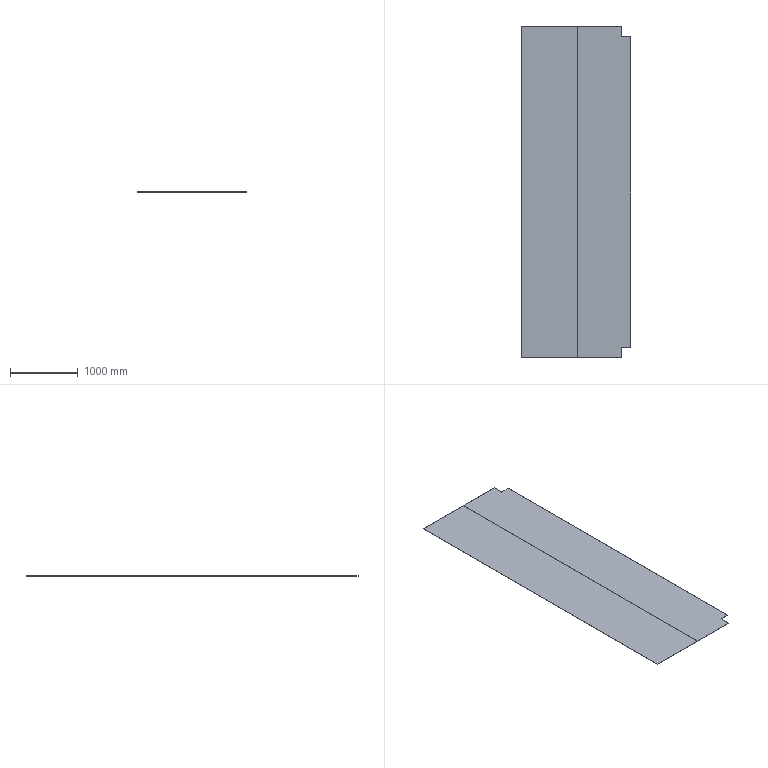Part | STEP file | 休息台花纹Plate 1 | 2 solids | 16 faces | box 1620 x 4900 x 3 mm | volume 23686830 mm3 | plane 16
STEP:
#1=CARTESIAN_POINT('',(0.,0.,0.));
#2=DIRECTION('',(0.,0.,1.));
#3=DIRECTION('',(1.,0.,0.));
#4=AXIS2_PLACEMENT_3D('',#1,#2,#3);
#5=CARTESIAN_POINT('',(1715.,50.,3.));
#6=VERTEX_POINT('',#5);
#7=CARTESIAN_POINT('',(1715.,50.,0.));
#8=VERTEX_POINT('',#7);
#9=CARTESIAN_POINT('',(1715.,50.,3.));
#10=DIRECTION('',(0.,0.,-1.));
#11=VECTOR('',#10,1.);
#12=LINE('',#9,#11);
#13=CARTESIAN_POINT('',(1715.,50.,-0.01));
#14=DIRECTION('',(-1.,0.,0.));
#15=DIRECTION('',(0.,-1.,0.));
#16=AXIS2_PLACEMENT_3D('',#13,#14,#15);
#17=PLANE('',#16);
#18=CARTESIAN_POINT('',(0.,3.01));
#19=DIRECTION('',(0.,-1.));
#20=VECTOR('',#19,1.);
#21=LINE('',#18,#20);
#22=(GEOMETRIC_REPRESENTATION_CONTEXT(2)PARAMETRIC_REPRESENTATION_CONTEXT()REPRESENTATION_CONTEXT('',''));
#23=DEFINITIONAL_REPRESENTATION('',(#21),#22);
#24=PCURVE('',#17,#23);
#25=CARTESIAN_POINT('',(2365.,50.,3.));
#26=DIRECTION('',(0.,-1.,0.));
#27=DIRECTION('',(0.,0.,-1.));
#28=AXIS2_PLACEMENT_3D('',#25,#26,#27);
#29=PLANE('',#28);
#30=CARTESIAN_POINT('',(0.,-650.));
#31=DIRECTION('',(1.,0.));
#32=VECTOR('',#31,1.);
#33=LINE('',#30,#32);
#34=(GEOMETRIC_REPRESENTATION_CONTEXT(2)PARAMETRIC_REPRESENTATION_CONTEXT()REPRESENTATION_CONTEXT('',''));
#35=DEFINITIONAL_REPRESENTATION('',(#33),#34);
#36=PCURVE('',#29,#35);
#37=SURFACE_CURVE('',#12,(#24,#36),.PCURVE_S1.);
#38=EDGE_CURVE('',#6,#8,#37,.T.);
#39=ORIENTED_EDGE('',*,*,#38,.F.);
#40=CARTESIAN_POINT('',(1715.,-4850.,3.));
#41=VERTEX_POINT('',#40);
#42=CARTESIAN_POINT('',(1715.,0.,3.));
#43=DIRECTION('',(0.,-1.,0.));
#44=VECTOR('',#43,1.);
#45=LINE('',#42,#44);
#46=CARTESIAN_POINT('',(50.,3.01));
#47=DIRECTION('',(1.,0.));
#48=VECTOR('',#47,1.);
#49=LINE('',#46,#48);
#50=(GEOMETRIC_REPRESENTATION_CONTEXT(2)PARAMETRIC_REPRESENTATION_CONTEXT()REPRESENTATION_CONTEXT('',''));
#51=DEFINITIONAL_REPRESENTATION('',(#49),#50);
#52=PCURVE('',#17,#51);
#53=CARTESIAN_POINT('',(0.,0.,3.));
#54=DIRECTION('',(0.,0.,1.));
#55=DIRECTION('',(1.,0.,0.));
#56=AXIS2_PLACEMENT_3D('',#53,#54,#55);
#57=PLANE('',#56);
#58=CARTESIAN_POINT('',(1715.,0.));
#59=DIRECTION('',(0.,-1.));
#60=VECTOR('',#59,1.);
#61=LINE('',#58,#60);
#62=(GEOMETRIC_REPRESENTATION_CONTEXT(2)PARAMETRIC_REPRESENTATION_CONTEXT()REPRESENTATION_CONTEXT('',''));
#63=DEFINITIONAL_REPRESENTATION('',(#61),#62);
#64=PCURVE('',#57,#63);
#65=SURFACE_CURVE('',#45,(#52,#64),.PCURVE_S1.);
#66=EDGE_CURVE('',#6,#41,#65,.T.);
#67=ORIENTED_EDGE('',*,*,#66,.T.);
#68=CARTESIAN_POINT('',(1715.,-4850.,0.));
#69=VERTEX_POINT('',#68);
#70=CARTESIAN_POINT('',(1715.,-4850.,3.));
#71=DIRECTION('',(0.,0.,1.));
#72=VECTOR('',#71,1.);
#73=LINE('',#70,#72);
#74=CARTESIAN_POINT('',(4900.,3.01));
#75=DIRECTION('',(0.,1.));
#76=VECTOR('',#75,1.);
#77=LINE('',#74,#76);
#78=(GEOMETRIC_REPRESENTATION_CONTEXT(2)PARAMETRIC_REPRESENTATION_CONTEXT()REPRESENTATION_CONTEXT('',''));
#79=DEFINITIONAL_REPRESENTATION('',(#77),#78);
#80=PCURVE('',#17,#79);
#81=CARTESIAN_POINT('',(880.,-4850.,3.));
#82=DIRECTION('',(0.,1.,0.));
#83=DIRECTION('',(0.,0.,1.));
#84=AXIS2_PLACEMENT_3D('',#81,#82,#83);
#85=PLANE('',#84);
#86=CARTESIAN_POINT('',(0.,835.));
#87=DIRECTION('',(1.,0.));
#88=VECTOR('',#87,1.);
#89=LINE('',#86,#88);
#90=(GEOMETRIC_REPRESENTATION_CONTEXT(2)PARAMETRIC_REPRESENTATION_CONTEXT()REPRESENTATION_CONTEXT('',''));
#91=DEFINITIONAL_REPRESENTATION('',(#89),#90);
#92=PCURVE('',#85,#91);
#93=SURFACE_CURVE('',#73,(#80,#92),.PCURVE_S1.);
#94=EDGE_CURVE('',#69,#41,#93,.T.);
#95=ORIENTED_EDGE('',*,*,#94,.F.);
#96=CARTESIAN_POINT('',(1715.,0.,0.));
#97=DIRECTION('',(0.,-1.,0.));
#98=VECTOR('',#97,1.);
#99=LINE('',#96,#98);
#100=CARTESIAN_POINT('',(50.,0.01));
#101=DIRECTION('',(1.,0.));
#102=VECTOR('',#101,1.);
#103=LINE('',#100,#102);
#104=(GEOMETRIC_REPRESENTATION_CONTEXT(2)PARAMETRIC_REPRESENTATION_CONTEXT()REPRESENTATION_CONTEXT('',''));
#105=DEFINITIONAL_REPRESENTATION('',(#103),#104);
#106=PCURVE('',#17,#105);
#107=CARTESIAN_POINT('',(0.,0.,0.));
#108=DIRECTION('',(0.,0.,1.));
#109=DIRECTION('',(1.,0.,0.));
#110=AXIS2_PLACEMENT_3D('',#107,#108,#109);
#111=PLANE('',#110);
#112=CARTESIAN_POINT('',(1715.,0.));
#113=DIRECTION('',(0.,-1.));
#114=VECTOR('',#113,1.);
#115=LINE('',#112,#114);
#116=(GEOMETRIC_REPRESENTATION_CONTEXT(2)PARAMETRIC_REPRESENTATION_CONTEXT()REPRESENTATION_CONTEXT('',''));
#117=DEFINITIONAL_REPRESENTATION('',(#115),#116);
#118=PCURVE('',#111,#117);
#119=SURFACE_CURVE('',#99,(#106,#118),.PCURVE_S1.);
#120=EDGE_CURVE('',#8,#69,#119,.T.);
#121=ORIENTED_EDGE('',*,*,#120,.F.);
#122=EDGE_LOOP('',(#39,#67,#95,#121));
#123=FACE_BOUND('',#122,.T.);
#124=ADVANCED_FACE('',(#123),#17,.F.);
#125=ORIENTED_EDGE('',*,*,#66,.F.);
#126=CARTESIAN_POINT('',(880.,50.,3.));
#127=VERTEX_POINT('',#126);
#128=CARTESIAN_POINT('',(2365.,50.,3.));
#129=DIRECTION('',(-1.,0.,0.));
#130=VECTOR('',#129,1.);
#131=LINE('',#128,#130);
#132=CARTESIAN_POINT('',(2365.,50.));
#133=DIRECTION('',(-1.,0.));
#134=VECTOR('',#133,1.);
#135=LINE('',#132,#134);
#136=(GEOMETRIC_REPRESENTATION_CONTEXT(2)PARAMETRIC_REPRESENTATION_CONTEXT()REPRESENTATION_CONTEXT('',''));
#137=DEFINITIONAL_REPRESENTATION('',(#135),#136);
#138=PCURVE('',#57,#137);
#139=CARTESIAN_POINT('',(0.,0.));
#140=DIRECTION('',(0.,-1.));
#141=VECTOR('',#140,1.);
#142=LINE('',#139,#141);
#143=(GEOMETRIC_REPRESENTATION_CONTEXT(2)PARAMETRIC_REPRESENTATION_CONTEXT()REPRESENTATION_CONTEXT('',''));
#144=DEFINITIONAL_REPRESENTATION('',(#142),#143);
#145=PCURVE('',#29,#144);
#146=SURFACE_CURVE('',#131,(#138,#145),.PCURVE_S1.);
#147=EDGE_CURVE('',#6,#127,#146,.T.);
#148=ORIENTED_EDGE('',*,*,#147,.T.);
#149=CARTESIAN_POINT('',(880.,-4850.,3.));
#150=VERTEX_POINT('',#149);
#151=CARTESIAN_POINT('',(880.,50.,3.));
#152=DIRECTION('',(0.,-1.,0.));
#153=VECTOR('',#152,1.);
#154=LINE('',#151,#153);
#155=CARTESIAN_POINT('',(880.,50.));
#156=DIRECTION('',(0.,-1.));
#157=VECTOR('',#156,1.);
#158=LINE('',#155,#157);
#159=(GEOMETRIC_REPRESENTATION_CONTEXT(2)PARAMETRIC_REPRESENTATION_CONTEXT()REPRESENTATION_CONTEXT('',''));
#160=DEFINITIONAL_REPRESENTATION('',(#158),#159);
#161=PCURVE('',#57,#160);
#162=CARTESIAN_POINT('',(880.,50.,3.));
#163=DIRECTION('',(1.,0.,0.));
#164=DIRECTION('',(0.,1.,0.));
#165=AXIS2_PLACEMENT_3D('',#162,#163,#164);
#166=PLANE('',#165);
#167=CARTESIAN_POINT('',(0.,0.));
#168=DIRECTION('',(-1.,0.));
#169=VECTOR('',#168,1.);
#170=LINE('',#167,#169);
#171=(GEOMETRIC_REPRESENTATION_CONTEXT(2)PARAMETRIC_REPRESENTATION_CONTEXT()REPRESENTATION_CONTEXT('',''));
#172=DEFINITIONAL_REPRESENTATION('',(#170),#171);
#173=PCURVE('',#166,#172);
#174=SURFACE_CURVE('',#154,(#161,#173),.PCURVE_S1.);
#175=EDGE_CURVE('',#127,#150,#174,.T.);
#176=ORIENTED_EDGE('',*,*,#175,.T.);
#177=CARTESIAN_POINT('',(880.,-4850.,3.));
#178=DIRECTION('',(1.,0.,0.));
#179=VECTOR('',#178,1.);
#180=LINE('',#177,#179);
#181=CARTESIAN_POINT('',(880.,-4850.));
#182=DIRECTION('',(1.,0.));
#183=VECTOR('',#182,1.);
#184=LINE('',#181,#183);
#185=(GEOMETRIC_REPRESENTATION_CONTEXT(2)PARAMETRIC_REPRESENTATION_CONTEXT()REPRESENTATION_CONTEXT('',''));
#186=DEFINITIONAL_REPRESENTATION('',(#184),#185);
#187=PCURVE('',#57,#186);
#188=CARTESIAN_POINT('',(0.,0.));
#189=DIRECTION('',(0.,1.));
#190=VECTOR('',#189,1.);
#191=LINE('',#188,#190);
#192=(GEOMETRIC_REPRESENTATION_CONTEXT(2)PARAMETRIC_REPRESENTATION_CONTEXT()REPRESENTATION_CONTEXT('',''));
#193=DEFINITIONAL_REPRESENTATION('',(#191),#192);
#194=PCURVE('',#85,#193);
#195=SURFACE_CURVE('',#180,(#187,#194),.PCURVE_S1.);
#196=EDGE_CURVE('',#150,#41,#195,.T.);
#197=ORIENTED_EDGE('',*,*,#196,.T.);
#198=EDGE_LOOP('',(#125,#148,#176,#197));
#199=FACE_BOUND('',#198,.T.);
#200=ADVANCED_FACE('',(#199),#57,.T.);
#201=CARTESIAN_POINT('',(880.,50.,0.));
#202=VERTEX_POINT('',#201);
#203=CARTESIAN_POINT('',(2365.,50.,0.));
#204=DIRECTION('',(-1.,0.,0.));
#205=VECTOR('',#204,1.);
#206=LINE('',#203,#205);
#207=CARTESIAN_POINT('',(2365.,50.));
#208=DIRECTION('',(-1.,0.));
#209=VECTOR('',#208,1.);
#210=LINE('',#207,#209);
#211=(GEOMETRIC_REPRESENTATION_CONTEXT(2)PARAMETRIC_REPRESENTATION_CONTEXT()REPRESENTATION_CONTEXT('',''));
#212=DEFINITIONAL_REPRESENTATION('',(#210),#211);
#213=PCURVE('',#111,#212);
#214=CARTESIAN_POINT('',(3.,0.));
#215=DIRECTION('',(0.,-1.));
#216=VECTOR('',#215,1.);
#217=LINE('',#214,#216);
#218=(GEOMETRIC_REPRESENTATION_CONTEXT(2)PARAMETRIC_REPRESENTATION_CONTEXT()REPRESENTATION_CONTEXT('',''));
#219=DEFINITIONAL_REPRESENTATION('',(#217),#218);
#220=PCURVE('',#29,#219);
#221=SURFACE_CURVE('',#206,(#213,#220),.PCURVE_S1.);
#222=EDGE_CURVE('',#8,#202,#221,.T.);
#223=ORIENTED_EDGE('',*,*,#222,.F.);
#224=ORIENTED_EDGE('',*,*,#120,.T.);
#225=CARTESIAN_POINT('',(880.,-4850.,0.));
#226=VERTEX_POINT('',#225);
#227=CARTESIAN_POINT('',(880.,-4850.,0.));
#228=DIRECTION('',(1.,0.,0.));
#229=VECTOR('',#228,1.);
#230=LINE('',#227,#229);
#231=CARTESIAN_POINT('',(880.,-4850.));
#232=DIRECTION('',(1.,0.));
#233=VECTOR('',#232,1.);
#234=LINE('',#231,#233);
#235=(GEOMETRIC_REPRESENTATION_CONTEXT(2)PARAMETRIC_REPRESENTATION_CONTEXT()REPRESENTATION_CONTEXT('',''));
#236=DEFINITIONAL_REPRESENTATION('',(#234),#235);
#237=PCURVE('',#111,#236);
#238=CARTESIAN_POINT('',(-3.,0.));
#239=DIRECTION('',(0.,1.));
#240=VECTOR('',#239,1.);
#241=LINE('',#238,#240);
#242=(GEOMETRIC_REPRESENTATION_CONTEXT(2)PARAMETRIC_REPRESENTATION_CONTEXT()REPRESENTATION_CONTEXT('',''));
#243=DEFINITIONAL_REPRESENTATION('',(#241),#242);
#244=PCURVE('',#85,#243);
#245=SURFACE_CURVE('',#230,(#237,#244),.PCURVE_S1.);
#246=EDGE_CURVE('',#226,#69,#245,.T.);
#247=ORIENTED_EDGE('',*,*,#246,.F.);
#248=CARTESIAN_POINT('',(880.,50.,0.));
#249=DIRECTION('',(0.,-1.,0.));
#250=VECTOR('',#249,1.);
#251=LINE('',#248,#250);
#252=CARTESIAN_POINT('',(880.,50.));
#253=DIRECTION('',(0.,-1.));
#254=VECTOR('',#253,1.);
#255=LINE('',#252,#254);
#256=(GEOMETRIC_REPRESENTATION_CONTEXT(2)PARAMETRIC_REPRESENTATION_CONTEXT()REPRESENTATION_CONTEXT('',''));
#257=DEFINITIONAL_REPRESENTATION('',(#255),#256);
#258=PCURVE('',#111,#257);
#259=CARTESIAN_POINT('',(0.,-3.));
#260=DIRECTION('',(-1.,0.));
#261=VECTOR('',#260,1.);
#262=LINE('',#259,#261);
#263=(GEOMETRIC_REPRESENTATION_CONTEXT(2)PARAMETRIC_REPRESENTATION_CONTEXT()REPRESENTATION_CONTEXT('',''));
#264=DEFINITIONAL_REPRESENTATION('',(#262),#263);
#265=PCURVE('',#166,#264);
#266=SURFACE_CURVE('',#251,(#258,#265),.PCURVE_S1.);
#267=EDGE_CURVE('',#202,#226,#266,.T.);
#268=ORIENTED_EDGE('',*,*,#267,.F.);
#269=EDGE_LOOP('',(#223,#224,#247,#268));
#270=FACE_BOUND('',#269,.T.);
#271=ADVANCED_FACE('',(#270),#111,.F.);
#272=ORIENTED_EDGE('',*,*,#147,.F.);
#273=ORIENTED_EDGE('',*,*,#38,.T.);
#274=ORIENTED_EDGE('',*,*,#222,.T.);
#275=CARTESIAN_POINT('',(880.,50.,3.));
#276=DIRECTION('',(0.,0.,-1.));
#277=VECTOR('',#276,1.);
#278=LINE('',#275,#277);
#279=CARTESIAN_POINT('',(0.,-1485.));
#280=DIRECTION('',(1.,0.));
#281=VECTOR('',#280,1.);
#282=LINE('',#279,#281);
#283=(GEOMETRIC_REPRESENTATION_CONTEXT(2)PARAMETRIC_REPRESENTATION_CONTEXT()REPRESENTATION_CONTEXT('',''));
#284=DEFINITIONAL_REPRESENTATION('',(#282),#283);
#285=PCURVE('',#29,#284);
#286=CARTESIAN_POINT('',(0.,0.));
#287=DIRECTION('',(0.,-1.));
#288=VECTOR('',#287,1.);
#289=LINE('',#286,#288);
#290=(GEOMETRIC_REPRESENTATION_CONTEXT(2)PARAMETRIC_REPRESENTATION_CONTEXT()REPRESENTATION_CONTEXT('',''));
#291=DEFINITIONAL_REPRESENTATION('',(#289),#290);
#292=PCURVE('',#166,#291);
#293=SURFACE_CURVE('',#278,(#285,#292),.PCURVE_S1.);
#294=EDGE_CURVE('',#127,#202,#293,.T.);
#295=ORIENTED_EDGE('',*,*,#294,.F.);
#296=EDGE_LOOP('',(#272,#273,#274,#295));
#297=FACE_BOUND('',#296,.T.);
#298=ADVANCED_FACE('',(#297),#29,.F.);
#299=ORIENTED_EDGE('',*,*,#246,.T.);
#300=ORIENTED_EDGE('',*,*,#94,.T.);
#301=ORIENTED_EDGE('',*,*,#196,.F.);
#302=CARTESIAN_POINT('',(880.,-4850.,3.));
#303=DIRECTION('',(0.,0.,-1.));
#304=VECTOR('',#303,1.);
#305=LINE('',#302,#304);
#306=CARTESIAN_POINT('',(0.,0.));
#307=DIRECTION('',(-1.,0.));
#308=VECTOR('',#307,1.);
#309=LINE('',#306,#308);
#310=(GEOMETRIC_REPRESENTATION_CONTEXT(2)PARAMETRIC_REPRESENTATION_CONTEXT()REPRESENTATION_CONTEXT('',''));
#311=DEFINITIONAL_REPRESENTATION('',(#309),#310);
#312=PCURVE('',#85,#311);
#313=CARTESIAN_POINT('',(-4900.,0.));
#314=DIRECTION('',(0.,-1.));
#315=VECTOR('',#314,1.);
#316=LINE('',#313,#315);
#317=(GEOMETRIC_REPRESENTATION_CONTEXT(2)PARAMETRIC_REPRESENTATION_CONTEXT()REPRESENTATION_CONTEXT('',''));
#318=DEFINITIONAL_REPRESENTATION('',(#316),#317);
#319=PCURVE('',#166,#318);
#320=SURFACE_CURVE('',#305,(#312,#319),.PCURVE_S1.);
#321=EDGE_CURVE('',#150,#226,#320,.T.);
#322=ORIENTED_EDGE('',*,*,#321,.T.);
#323=EDGE_LOOP('',(#299,#300,#301,#322));
#324=FACE_BOUND('',#323,.T.);
#325=ADVANCED_FACE('',(#324),#85,.F.);
#326=ORIENTED_EDGE('',*,*,#267,.T.);
#327=ORIENTED_EDGE('',*,*,#321,.F.);
#328=ORIENTED_EDGE('',*,*,#175,.F.);
#329=ORIENTED_EDGE('',*,*,#294,.T.);
#330=EDGE_LOOP('',(#326,#327,#328,#329));
#331=FACE_BOUND('',#330,.T.);
#332=ADVANCED_FACE('',(#331),#166,.F.);
#333=CLOSED_SHELL('',(#124,#200,#271,#298,#325,#332));
#334=MANIFOLD_SOLID_BREP('',#333);
#335=CARTESIAN_POINT('',(1715.,50.,3.));
#336=VERTEX_POINT('',#335);
#337=CARTESIAN_POINT('',(1715.,50.,0.));
#338=VERTEX_POINT('',#337);
#339=CARTESIAN_POINT('',(1715.,50.,3.));
#340=DIRECTION('',(0.,0.,-1.));
#341=VECTOR('',#340,1.);
#342=LINE('',#339,#341);
#343=CARTESIAN_POINT('',(2365.,50.,3.));
#344=DIRECTION('',(0.,-1.,0.));
#345=DIRECTION('',(0.,0.,-1.));
#346=AXIS2_PLACEMENT_3D('',#343,#344,#345);
#347=PLANE('',#346);
#348=CARTESIAN_POINT('',(0.,-650.));
#349=DIRECTION('',(1.,0.));
#350=VECTOR('',#349,1.);
#351=LINE('',#348,#350);
#352=(GEOMETRIC_REPRESENTATION_CONTEXT(2)PARAMETRIC_REPRESENTATION_CONTEXT()REPRESENTATION_CONTEXT('',''));
#353=DEFINITIONAL_REPRESENTATION('',(#351),#352);
#354=PCURVE('',#347,#353);
#355=CARTESIAN_POINT('',(1715.,50.,-0.01));
#356=DIRECTION('',(-1.,0.,0.));
#357=DIRECTION('',(0.,-1.,0.));
#358=AXIS2_PLACEMENT_3D('',#355,#356,#357);
#359=PLANE('',#358);
#360=CARTESIAN_POINT('',(0.,3.01));
#361=DIRECTION('',(0.,-1.));
#362=VECTOR('',#361,1.);
#363=LINE('',#360,#362);
#364=(GEOMETRIC_REPRESENTATION_CONTEXT(2)PARAMETRIC_REPRESENTATION_CONTEXT()REPRESENTATION_CONTEXT('',''));
#365=DEFINITIONAL_REPRESENTATION('',(#363),#364);
#366=PCURVE('',#359,#365);
#367=SURFACE_CURVE('',#342,(#354,#366),.PCURVE_S1.);
#368=EDGE_CURVE('',#336,#338,#367,.T.);
#369=ORIENTED_EDGE('',*,*,#368,.F.);
#370=CARTESIAN_POINT('',(2365.,50.,3.));
#371=VERTEX_POINT('',#370);
#372=CARTESIAN_POINT('',(2365.,50.,3.));
#373=DIRECTION('',(-1.,0.,0.));
#374=VECTOR('',#373,1.);
#375=LINE('',#372,#374);
#376=CARTESIAN_POINT('',(0.,0.));
#377=DIRECTION('',(0.,-1.));
#378=VECTOR('',#377,1.);
#379=LINE('',#376,#378);
#380=(GEOMETRIC_REPRESENTATION_CONTEXT(2)PARAMETRIC_REPRESENTATION_CONTEXT()REPRESENTATION_CONTEXT('',''));
#381=DEFINITIONAL_REPRESENTATION('',(#379),#380);
#382=PCURVE('',#347,#381);
#383=CARTESIAN_POINT('',(0.,0.,3.));
#384=DIRECTION('',(0.,0.,1.));
#385=DIRECTION('',(1.,0.,0.));
#386=AXIS2_PLACEMENT_3D('',#383,#384,#385);
#387=PLANE('',#386);
#388=CARTESIAN_POINT('',(2365.,50.));
#389=DIRECTION('',(-1.,0.));
#390=VECTOR('',#389,1.);
#391=LINE('',#388,#390);
#392=(GEOMETRIC_REPRESENTATION_CONTEXT(2)PARAMETRIC_REPRESENTATION_CONTEXT()REPRESENTATION_CONTEXT('',''));
#393=DEFINITIONAL_REPRESENTATION('',(#391),#392);
#394=PCURVE('',#387,#393);
#395=SURFACE_CURVE('',#375,(#382,#394),.PCURVE_S1.);
#396=EDGE_CURVE('',#371,#336,#395,.T.);
#397=ORIENTED_EDGE('',*,*,#396,.F.);
#398=CARTESIAN_POINT('',(2365.,50.,0.));
#399=VERTEX_POINT('',#398);
#400=CARTESIAN_POINT('',(2365.,50.,3.));
#401=DIRECTION('',(0.,0.,-1.));
#402=VECTOR('',#401,1.);
#403=LINE('',#400,#402);
#404=CARTESIAN_POINT('',(0.,0.));
#405=DIRECTION('',(1.,0.));
#406=VECTOR('',#405,1.);
#407=LINE('',#404,#406);
#408=(GEOMETRIC_REPRESENTATION_CONTEXT(2)PARAMETRIC_REPRESENTATION_CONTEXT()REPRESENTATION_CONTEXT('',''));
#409=DEFINITIONAL_REPRESENTATION('',(#407),#408);
#410=PCURVE('',#347,#409);
#411=CARTESIAN_POINT('',(2365.,-107.,3.));
#412=DIRECTION('',(-1.,0.,0.));
#413=DIRECTION('',(0.,0.,1.));
#414=AXIS2_PLACEMENT_3D('',#411,#412,#413);
#415=PLANE('',#414);
#416=CARTESIAN_POINT('',(0.,157.));
#417=DIRECTION('',(-1.,0.));
#418=VECTOR('',#417,1.);
#419=LINE('',#416,#418);
#420=(GEOMETRIC_REPRESENTATION_CONTEXT(2)PARAMETRIC_REPRESENTATION_CONTEXT()REPRESENTATION_CONTEXT('',''));
#421=DEFINITIONAL_REPRESENTATION('',(#419),#420);
#422=PCURVE('',#415,#421);
#423=SURFACE_CURVE('',#403,(#410,#422),.PCURVE_S1.);
#424=EDGE_CURVE('',#371,#399,#423,.T.);
#425=ORIENTED_EDGE('',*,*,#424,.T.);
#426=CARTESIAN_POINT('',(2365.,50.,0.));
#427=DIRECTION('',(-1.,0.,0.));
#428=VECTOR('',#427,1.);
#429=LINE('',#426,#428);
#430=CARTESIAN_POINT('',(3.,0.));
#431=DIRECTION('',(0.,-1.));
#432=VECTOR('',#431,1.);
#433=LINE('',#430,#432);
#434=(GEOMETRIC_REPRESENTATION_CONTEXT(2)PARAMETRIC_REPRESENTATION_CONTEXT()REPRESENTATION_CONTEXT('',''));
#435=DEFINITIONAL_REPRESENTATION('',(#433),#434);
#436=PCURVE('',#347,#435);
#437=CARTESIAN_POINT('',(0.,0.,0.));
#438=DIRECTION('',(0.,0.,1.));
#439=DIRECTION('',(1.,0.,0.));
#440=AXIS2_PLACEMENT_3D('',#437,#438,#439);
#441=PLANE('',#440);
#442=CARTESIAN_POINT('',(2365.,50.));
#443=DIRECTION('',(-1.,0.));
#444=VECTOR('',#443,1.);
#445=LINE('',#442,#444);
#446=(GEOMETRIC_REPRESENTATION_CONTEXT(2)PARAMETRIC_REPRESENTATION_CONTEXT()REPRESENTATION_CONTEXT('',''));
#447=DEFINITIONAL_REPRESENTATION('',(#445),#446);
#448=PCURVE('',#441,#447);
#449=SURFACE_CURVE('',#429,(#436,#448),.PCURVE_S1.);
#450=EDGE_CURVE('',#399,#338,#449,.T.);
#451=ORIENTED_EDGE('',*,*,#450,.T.);
#452=EDGE_LOOP('',(#369,#397,#425,#451));
#453=FACE_BOUND('',#452,.T.);
#454=ADVANCED_FACE('',(#453),#347,.F.);
#455=CARTESIAN_POINT('',(1715.,-4850.,0.));
#456=VERTEX_POINT('',#455);
#457=CARTESIAN_POINT('',(1715.,-4850.,3.));
#458=VERTEX_POINT('',#457);
#459=CARTESIAN_POINT('',(1715.,-4850.,3.));
#460=DIRECTION('',(0.,0.,1.));
#461=VECTOR('',#460,1.);
#462=LINE('',#459,#461);
#463=CARTESIAN_POINT('',(880.,-4850.,3.));
#464=DIRECTION('',(0.,1.,0.));
#465=DIRECTION('',(0.,0.,1.));
#466=AXIS2_PLACEMENT_3D('',#463,#464,#465);
#467=PLANE('',#466);
#468=CARTESIAN_POINT('',(0.,835.));
#469=DIRECTION('',(1.,0.));
#470=VECTOR('',#469,1.);
#471=LINE('',#468,#470);
#472=(GEOMETRIC_REPRESENTATION_CONTEXT(2)PARAMETRIC_REPRESENTATION_CONTEXT()REPRESENTATION_CONTEXT('',''));
#473=DEFINITIONAL_REPRESENTATION('',(#471),#472);
#474=PCURVE('',#467,#473);
#475=CARTESIAN_POINT('',(4900.,3.01));
#476=DIRECTION('',(0.,1.));
#477=VECTOR('',#476,1.);
#478=LINE('',#475,#477);
#479=(GEOMETRIC_REPRESENTATION_CONTEXT(2)PARAMETRIC_REPRESENTATION_CONTEXT()REPRESENTATION_CONTEXT('',''));
#480=DEFINITIONAL_REPRESENTATION('',(#478),#479);
#481=PCURVE('',#359,#480);
#482=SURFACE_CURVE('',#462,(#474,#481),.PCURVE_S1.);
#483=EDGE_CURVE('',#456,#458,#482,.T.);
#484=ORIENTED_EDGE('',*,*,#483,.F.);
#485=CARTESIAN_POINT('',(2365.,-4850.,0.));
#486=VERTEX_POINT('',#485);
#487=CARTESIAN_POINT('',(880.,-4850.,0.));
#488=DIRECTION('',(1.,0.,0.));
#489=VECTOR('',#488,1.);
#490=LINE('',#487,#489);
#491=CARTESIAN_POINT('',(-3.,0.));
#492=DIRECTION('',(0.,1.));
#493=VECTOR('',#492,1.);
#494=LINE('',#491,#493);
#495=(GEOMETRIC_REPRESENTATION_CONTEXT(2)PARAMETRIC_REPRESENTATION_CONTEXT()REPRESENTATION_CONTEXT('',''));
#496=DEFINITIONAL_REPRESENTATION('',(#494),#495);
#497=PCURVE('',#467,#496);
#498=CARTESIAN_POINT('',(880.,-4850.));
#499=DIRECTION('',(1.,0.));
#500=VECTOR('',#499,1.);
#501=LINE('',#498,#500);
#502=(GEOMETRIC_REPRESENTATION_CONTEXT(2)PARAMETRIC_REPRESENTATION_CONTEXT()REPRESENTATION_CONTEXT('',''));
#503=DEFINITIONAL_REPRESENTATION('',(#501),#502);
#504=PCURVE('',#441,#503);
#505=SURFACE_CURVE('',#490,(#497,#504),.PCURVE_S1.);
#506=EDGE_CURVE('',#456,#486,#505,.T.);
#507=ORIENTED_EDGE('',*,*,#506,.T.);
#508=CARTESIAN_POINT('',(2365.,-4850.,3.));
#509=VERTEX_POINT('',#508);
#510=CARTESIAN_POINT('',(2365.,-4850.,3.));
#511=DIRECTION('',(0.,0.,-1.));
#512=VECTOR('',#511,1.);
#513=LINE('',#510,#512);
#514=CARTESIAN_POINT('',(0.,1485.));
#515=DIRECTION('',(-1.,0.));
#516=VECTOR('',#515,1.);
#517=LINE('',#514,#516);
#518=(GEOMETRIC_REPRESENTATION_CONTEXT(2)PARAMETRIC_REPRESENTATION_CONTEXT()REPRESENTATION_CONTEXT('',''));
#519=DEFINITIONAL_REPRESENTATION('',(#517),#518);
#520=PCURVE('',#467,#519);
#521=CARTESIAN_POINT('',(2365.,-4850.,3.));
#522=DIRECTION('',(-1.,0.,0.));
#523=DIRECTION('',(0.,0.,1.));
#524=AXIS2_PLACEMENT_3D('',#521,#522,#523);
#525=PLANE('',#524);
#526=CARTESIAN_POINT('',(0.,0.));
#527=DIRECTION('',(-1.,0.));
#528=VECTOR('',#527,1.);
#529=LINE('',#526,#528);
#530=(GEOMETRIC_REPRESENTATION_CONTEXT(2)PARAMETRIC_REPRESENTATION_CONTEXT()REPRESENTATION_CONTEXT('',''));
#531=DEFINITIONAL_REPRESENTATION('',(#529),#530);
#532=PCURVE('',#525,#531);
#533=SURFACE_CURVE('',#513,(#520,#532),.PCURVE_S1.);
#534=EDGE_CURVE('',#509,#486,#533,.T.);
#535=ORIENTED_EDGE('',*,*,#534,.F.);
#536=CARTESIAN_POINT('',(880.,-4850.,3.));
#537=DIRECTION('',(1.,0.,0.));
#538=VECTOR('',#537,1.);
#539=LINE('',#536,#538);
#540=CARTESIAN_POINT('',(0.,0.));
#541=DIRECTION('',(0.,1.));
#542=VECTOR('',#541,1.);
#543=LINE('',#540,#542);
#544=(GEOMETRIC_REPRESENTATION_CONTEXT(2)PARAMETRIC_REPRESENTATION_CONTEXT()REPRESENTATION_CONTEXT('',''));
#545=DEFINITIONAL_REPRESENTATION('',(#543),#544);
#546=PCURVE('',#467,#545);
#547=CARTESIAN_POINT('',(880.,-4850.));
#548=DIRECTION('',(1.,0.));
#549=VECTOR('',#548,1.);
#550=LINE('',#547,#549);
#551=(GEOMETRIC_REPRESENTATION_CONTEXT(2)PARAMETRIC_REPRESENTATION_CONTEXT()REPRESENTATION_CONTEXT('',''));
#552=DEFINITIONAL_REPRESENTATION('',(#550),#551);
#553=PCURVE('',#387,#552);
#554=SURFACE_CURVE('',#539,(#546,#553),.PCURVE_S1.);
#555=EDGE_CURVE('',#458,#509,#554,.T.);
#556=ORIENTED_EDGE('',*,*,#555,.F.);
#557=EDGE_LOOP('',(#484,#507,#535,#556));
#558=FACE_BOUND('',#557,.T.);
#559=ADVANCED_FACE('',(#558),#467,.F.);
#560=ORIENTED_EDGE('',*,*,#396,.T.);
#561=CARTESIAN_POINT('',(1715.,0.,3.));
#562=DIRECTION('',(0.,-1.,0.));
#563=VECTOR('',#562,1.);
#564=LINE('',#561,#563);
#565=CARTESIAN_POINT('',(1715.,0.));
#566=DIRECTION('',(0.,-1.));
#567=VECTOR('',#566,1.);
#568=LINE('',#565,#567);
#569=(GEOMETRIC_REPRESENTATION_CONTEXT(2)PARAMETRIC_REPRESENTATION_CONTEXT()REPRESENTATION_CONTEXT('',''));
#570=DEFINITIONAL_REPRESENTATION('',(#568),#569);
#571=PCURVE('',#387,#570);
#572=CARTESIAN_POINT('',(50.,3.01));
#573=DIRECTION('',(1.,0.));
#574=VECTOR('',#573,1.);
#575=LINE('',#572,#574);
#576=(GEOMETRIC_REPRESENTATION_CONTEXT(2)PARAMETRIC_REPRESENTATION_CONTEXT()REPRESENTATION_CONTEXT('',''));
#577=DEFINITIONAL_REPRESENTATION('',(#575),#576);
#578=PCURVE('',#359,#577);
#579=SURFACE_CURVE('',#564,(#571,#578),.PCURVE_S1.);
#580=EDGE_CURVE('',#336,#458,#579,.T.);
#581=ORIENTED_EDGE('',*,*,#580,.T.);
#582=ORIENTED_EDGE('',*,*,#555,.T.);
#583=CARTESIAN_POINT('',(2365.,-4693.,3.));
#584=VERTEX_POINT('',#583);
#585=CARTESIAN_POINT('',(2365.,-4850.,3.));
#586=DIRECTION('',(0.,1.,0.));
#587=VECTOR('',#586,1.);
#588=LINE('',#585,#587);
#589=CARTESIAN_POINT('',(2365.,-4850.));
#590=DIRECTION('',(0.,1.));
#591=VECTOR('',#590,1.);
#592=LINE('',#589,#591);
#593=(GEOMETRIC_REPRESENTATION_CONTEXT(2)PARAMETRIC_REPRESENTATION_CONTEXT()REPRESENTATION_CONTEXT('',''));
#594=DEFINITIONAL_REPRESENTATION('',(#592),#593);
#595=PCURVE('',#387,#594);
#596=CARTESIAN_POINT('',(0.,0.));
#597=DIRECTION('',(0.,1.));
#598=VECTOR('',#597,1.);
#599=LINE('',#596,#598);
#600=(GEOMETRIC_REPRESENTATION_CONTEXT(2)PARAMETRIC_REPRESENTATION_CONTEXT()REPRESENTATION_CONTEXT('',''));
#601=DEFINITIONAL_REPRESENTATION('',(#599),#600);
#602=PCURVE('',#525,#601);
#603=SURFACE_CURVE('',#588,(#595,#602),.PCURVE_S1.);
#604=EDGE_CURVE('',#509,#584,#603,.T.);
#605=ORIENTED_EDGE('',*,*,#604,.T.);
#606=CARTESIAN_POINT('',(2500.,-4693.,3.));
#607=VERTEX_POINT('',#606);
#608=CARTESIAN_POINT('',(2365.,-4693.,3.));
#609=DIRECTION('',(1.,0.,0.));
#610=VECTOR('',#609,1.);
#611=LINE('',#608,#610);
#612=CARTESIAN_POINT('',(2365.,-4693.));
#613=DIRECTION('',(1.,0.));
#614=VECTOR('',#613,1.);
#615=LINE('',#612,#614);
#616=(GEOMETRIC_REPRESENTATION_CONTEXT(2)PARAMETRIC_REPRESENTATION_CONTEXT()REPRESENTATION_CONTEXT('',''));
#617=DEFINITIONAL_REPRESENTATION('',(#615),#616);
#618=PCURVE('',#387,#617);
#619=CARTESIAN_POINT('',(2365.,-4693.,3.));
#620=DIRECTION('',(0.,1.,0.));
#621=DIRECTION('',(0.,0.,1.));
#622=AXIS2_PLACEMENT_3D('',#619,#620,#621);
#623=PLANE('',#622);
#624=CARTESIAN_POINT('',(0.,0.));
#625=DIRECTION('',(0.,1.));
#626=VECTOR('',#625,1.);
#627=LINE('',#624,#626);
#628=(GEOMETRIC_REPRESENTATION_CONTEXT(2)PARAMETRIC_REPRESENTATION_CONTEXT()REPRESENTATION_CONTEXT('',''));
#629=DEFINITIONAL_REPRESENTATION('',(#627),#628);
#630=PCURVE('',#623,#629);
#631=SURFACE_CURVE('',#611,(#618,#630),.PCURVE_S1.);
#632=EDGE_CURVE('',#584,#607,#631,.T.);
#633=ORIENTED_EDGE('',*,*,#632,.T.);
#634=CARTESIAN_POINT('',(2500.,-107.,3.));
#635=VERTEX_POINT('',#634);
#636=CARTESIAN_POINT('',(2500.,-4693.,3.));
#637=DIRECTION('',(0.,1.,0.));
#638=VECTOR('',#637,1.);
#639=LINE('',#636,#638);
#640=CARTESIAN_POINT('',(2500.,-4693.));
#641=DIRECTION('',(0.,1.));
#642=VECTOR('',#641,1.);
#643=LINE('',#640,#642);
#644=(GEOMETRIC_REPRESENTATION_CONTEXT(2)PARAMETRIC_REPRESENTATION_CONTEXT()REPRESENTATION_CONTEXT('',''));
#645=DEFINITIONAL_REPRESENTATION('',(#643),#644);
#646=PCURVE('',#387,#645);
#647=CARTESIAN_POINT('',(2500.,-4693.,3.));
#648=DIRECTION('',(-1.,0.,0.));
#649=DIRECTION('',(0.,-1.,0.));
#650=AXIS2_PLACEMENT_3D('',#647,#648,#649);
#651=PLANE('',#650);
#652=CARTESIAN_POINT('',(0.,0.));
#653=DIRECTION('',(-1.,0.));
#654=VECTOR('',#653,1.);
#655=LINE('',#652,#654);
#656=(GEOMETRIC_REPRESENTATION_CONTEXT(2)PARAMETRIC_REPRESENTATION_CONTEXT()REPRESENTATION_CONTEXT('',''));
#657=DEFINITIONAL_REPRESENTATION('',(#655),#656);
#658=PCURVE('',#651,#657);
#659=SURFACE_CURVE('',#639,(#646,#658),.PCURVE_S1.);
#660=EDGE_CURVE('',#607,#635,#659,.T.);
#661=ORIENTED_EDGE('',*,*,#660,.T.);
#662=CARTESIAN_POINT('',(2365.,-107.,3.));
#663=VERTEX_POINT('',#662);
#664=CARTESIAN_POINT('',(2500.,-107.,3.));
#665=DIRECTION('',(-1.,0.,0.));
#666=VECTOR('',#665,1.);
#667=LINE('',#664,#666);
#668=CARTESIAN_POINT('',(2500.,-107.));
#669=DIRECTION('',(-1.,0.));
#670=VECTOR('',#669,1.);
#671=LINE('',#668,#670);
#672=(GEOMETRIC_REPRESENTATION_CONTEXT(2)PARAMETRIC_REPRESENTATION_CONTEXT()REPRESENTATION_CONTEXT('',''));
#673=DEFINITIONAL_REPRESENTATION('',(#671),#672);
#674=PCURVE('',#387,#673);
#675=CARTESIAN_POINT('',(2500.,-107.,3.));
#676=DIRECTION('',(0.,-1.,0.));
#677=DIRECTION('',(0.,0.,-1.));
#678=AXIS2_PLACEMENT_3D('',#675,#676,#677);
#679=PLANE('',#678);
#680=CARTESIAN_POINT('',(0.,0.));
#681=DIRECTION('',(0.,-1.));
#682=VECTOR('',#681,1.);
#683=LINE('',#680,#682);
#684=(GEOMETRIC_REPRESENTATION_CONTEXT(2)PARAMETRIC_REPRESENTATION_CONTEXT()REPRESENTATION_CONTEXT('',''));
#685=DEFINITIONAL_REPRESENTATION('',(#683),#684);
#686=PCURVE('',#679,#685);
#687=SURFACE_CURVE('',#667,(#674,#686),.PCURVE_S1.);
#688=EDGE_CURVE('',#635,#663,#687,.T.);
#689=ORIENTED_EDGE('',*,*,#688,.T.);
#690=CARTESIAN_POINT('',(2365.,-107.,3.));
#691=DIRECTION('',(0.,1.,0.));
#692=VECTOR('',#691,1.);
#693=LINE('',#690,#692);
#694=CARTESIAN_POINT('',(2365.,-107.));
#695=DIRECTION('',(0.,1.));
#696=VECTOR('',#695,1.);
#697=LINE('',#694,#696);
#698=(GEOMETRIC_REPRESENTATION_CONTEXT(2)PARAMETRIC_REPRESENTATION_CONTEXT()REPRESENTATION_CONTEXT('',''));
#699=DEFINITIONAL_REPRESENTATION('',(#697),#698);
#700=PCURVE('',#387,#699);
#701=CARTESIAN_POINT('',(0.,0.));
#702=DIRECTION('',(0.,1.));
#703=VECTOR('',#702,1.);
#704=LINE('',#701,#703);
#705=(GEOMETRIC_REPRESENTATION_CONTEXT(2)PARAMETRIC_REPRESENTATION_CONTEXT()REPRESENTATION_CONTEXT('',''));
#706=DEFINITIONAL_REPRESENTATION('',(#704),#705);
#707=PCURVE('',#415,#706);
#708=SURFACE_CURVE('',#693,(#700,#707),.PCURVE_S1.);
#709=EDGE_CURVE('',#663,#371,#708,.T.);
#710=ORIENTED_EDGE('',*,*,#709,.T.);
#711=EDGE_LOOP('',(#560,#581,#582,#605,#633,#661,#689,#710));
#712=FACE_BOUND('',#711,.T.);
#713=ADVANCED_FACE('',(#712),#387,.T.);
#714=CARTESIAN_POINT('',(1715.,0.,0.));
#715=DIRECTION('',(0.,-1.,0.));
#716=VECTOR('',#715,1.);
#717=LINE('',#714,#716);
#718=CARTESIAN_POINT('',(1715.,0.));
#719=DIRECTION('',(0.,-1.));
#720=VECTOR('',#719,1.);
#721=LINE('',#718,#720);
#722=(GEOMETRIC_REPRESENTATION_CONTEXT(2)PARAMETRIC_REPRESENTATION_CONTEXT()REPRESENTATION_CONTEXT('',''));
#723=DEFINITIONAL_REPRESENTATION('',(#721),#722);
#724=PCURVE('',#441,#723);
#725=CARTESIAN_POINT('',(50.,0.01));
#726=DIRECTION('',(1.,0.));
#727=VECTOR('',#726,1.);
#728=LINE('',#725,#727);
#729=(GEOMETRIC_REPRESENTATION_CONTEXT(2)PARAMETRIC_REPRESENTATION_CONTEXT()REPRESENTATION_CONTEXT('',''));
#730=DEFINITIONAL_REPRESENTATION('',(#728),#729);
#731=PCURVE('',#359,#730);
#732=SURFACE_CURVE('',#717,(#724,#731),.PCURVE_S1.);
#733=EDGE_CURVE('',#338,#456,#732,.T.);
#734=ORIENTED_EDGE('',*,*,#733,.F.);
#735=ORIENTED_EDGE('',*,*,#450,.F.);
#736=CARTESIAN_POINT('',(2365.,-107.,0.));
#737=VERTEX_POINT('',#736);
#738=CARTESIAN_POINT('',(2365.,-107.,0.));
#739=DIRECTION('',(0.,1.,0.));
#740=VECTOR('',#739,1.);
#741=LINE('',#738,#740);
#742=CARTESIAN_POINT('',(2365.,-107.));
#743=DIRECTION('',(0.,1.));
#744=VECTOR('',#743,1.);
#745=LINE('',#742,#744);
#746=(GEOMETRIC_REPRESENTATION_CONTEXT(2)PARAMETRIC_REPRESENTATION_CONTEXT()REPRESENTATION_CONTEXT('',''));
#747=DEFINITIONAL_REPRESENTATION('',(#745),#746);
#748=PCURVE('',#441,#747);
#749=CARTESIAN_POINT('',(-3.,0.));
#750=DIRECTION('',(0.,1.));
#751=VECTOR('',#750,1.);
#752=LINE('',#749,#751);
#753=(GEOMETRIC_REPRESENTATION_CONTEXT(2)PARAMETRIC_REPRESENTATION_CONTEXT()REPRESENTATION_CONTEXT('',''));
#754=DEFINITIONAL_REPRESENTATION('',(#752),#753);
#755=PCURVE('',#415,#754);
#756=SURFACE_CURVE('',#741,(#748,#755),.PCURVE_S1.);
#757=EDGE_CURVE('',#737,#399,#756,.T.);
#758=ORIENTED_EDGE('',*,*,#757,.F.);
#759=CARTESIAN_POINT('',(2500.,-107.,0.));
#760=VERTEX_POINT('',#759);
#761=CARTESIAN_POINT('',(2500.,-107.,0.));
#762=DIRECTION('',(-1.,0.,0.));
#763=VECTOR('',#762,1.);
#764=LINE('',#761,#763);
#765=CARTESIAN_POINT('',(2500.,-107.));
#766=DIRECTION('',(-1.,0.));
#767=VECTOR('',#766,1.);
#768=LINE('',#765,#767);
#769=(GEOMETRIC_REPRESENTATION_CONTEXT(2)PARAMETRIC_REPRESENTATION_CONTEXT()REPRESENTATION_CONTEXT('',''));
#770=DEFINITIONAL_REPRESENTATION('',(#768),#769);
#771=PCURVE('',#441,#770);
#772=CARTESIAN_POINT('',(3.,0.));
#773=DIRECTION('',(0.,-1.));
#774=VECTOR('',#773,1.);
#775=LINE('',#772,#774);
#776=(GEOMETRIC_REPRESENTATION_CONTEXT(2)PARAMETRIC_REPRESENTATION_CONTEXT()REPRESENTATION_CONTEXT('',''));
#777=DEFINITIONAL_REPRESENTATION('',(#775),#776);
#778=PCURVE('',#679,#777);
#779=SURFACE_CURVE('',#764,(#771,#778),.PCURVE_S1.);
#780=EDGE_CURVE('',#760,#737,#779,.T.);
#781=ORIENTED_EDGE('',*,*,#780,.F.);
#782=CARTESIAN_POINT('',(2500.,-4693.,0.));
#783=VERTEX_POINT('',#782);
#784=CARTESIAN_POINT('',(2500.,-4693.,0.));
#785=DIRECTION('',(0.,1.,0.));
#786=VECTOR('',#785,1.);
#787=LINE('',#784,#786);
#788=CARTESIAN_POINT('',(2500.,-4693.));
#789=DIRECTION('',(0.,1.));
#790=VECTOR('',#789,1.);
#791=LINE('',#788,#790);
#792=(GEOMETRIC_REPRESENTATION_CONTEXT(2)PARAMETRIC_REPRESENTATION_CONTEXT()REPRESENTATION_CONTEXT('',''));
#793=DEFINITIONAL_REPRESENTATION('',(#791),#792);
#794=PCURVE('',#441,#793);
#795=CARTESIAN_POINT('',(0.,-3.));
#796=DIRECTION('',(-1.,0.));
#797=VECTOR('',#796,1.);
#798=LINE('',#795,#797);
#799=(GEOMETRIC_REPRESENTATION_CONTEXT(2)PARAMETRIC_REPRESENTATION_CONTEXT()REPRESENTATION_CONTEXT('',''));
#800=DEFINITIONAL_REPRESENTATION('',(#798),#799);
#801=PCURVE('',#651,#800);
#802=SURFACE_CURVE('',#787,(#794,#801),.PCURVE_S1.);
#803=EDGE_CURVE('',#783,#760,#802,.T.);
#804=ORIENTED_EDGE('',*,*,#803,.F.);
#805=CARTESIAN_POINT('',(2365.,-4693.,0.));
#806=VERTEX_POINT('',#805);
#807=CARTESIAN_POINT('',(2365.,-4693.,0.));
#808=DIRECTION('',(1.,0.,0.));
#809=VECTOR('',#808,1.);
#810=LINE('',#807,#809);
#811=CARTESIAN_POINT('',(2365.,-4693.));
#812=DIRECTION('',(1.,0.));
#813=VECTOR('',#812,1.);
#814=LINE('',#811,#813);
#815=(GEOMETRIC_REPRESENTATION_CONTEXT(2)PARAMETRIC_REPRESENTATION_CONTEXT()REPRESENTATION_CONTEXT('',''));
#816=DEFINITIONAL_REPRESENTATION('',(#814),#815);
#817=PCURVE('',#441,#816);
#818=CARTESIAN_POINT('',(-3.,0.));
#819=DIRECTION('',(0.,1.));
#820=VECTOR('',#819,1.);
#821=LINE('',#818,#820);
#822=(GEOMETRIC_REPRESENTATION_CONTEXT(2)PARAMETRIC_REPRESENTATION_CONTEXT()REPRESENTATION_CONTEXT('',''));
#823=DEFINITIONAL_REPRESENTATION('',(#821),#822);
#824=PCURVE('',#623,#823);
#825=SURFACE_CURVE('',#810,(#817,#824),.PCURVE_S1.);
#826=EDGE_CURVE('',#806,#783,#825,.T.);
#827=ORIENTED_EDGE('',*,*,#826,.F.);
#828=CARTESIAN_POINT('',(2365.,-4850.,0.));
#829=DIRECTION('',(0.,1.,0.));
#830=VECTOR('',#829,1.);
#831=LINE('',#828,#830);
#832=CARTESIAN_POINT('',(2365.,-4850.));
#833=DIRECTION('',(0.,1.));
#834=VECTOR('',#833,1.);
#835=LINE('',#832,#834);
#836=(GEOMETRIC_REPRESENTATION_CONTEXT(2)PARAMETRIC_REPRESENTATION_CONTEXT()REPRESENTATION_CONTEXT('',''));
#837=DEFINITIONAL_REPRESENTATION('',(#835),#836);
#838=PCURVE('',#441,#837);
#839=CARTESIAN_POINT('',(-3.,0.));
#840=DIRECTION('',(0.,1.));
#841=VECTOR('',#840,1.);
#842=LINE('',#839,#841);
#843=(GEOMETRIC_REPRESENTATION_CONTEXT(2)PARAMETRIC_REPRESENTATION_CONTEXT()REPRESENTATION_CONTEXT('',''));
#844=DEFINITIONAL_REPRESENTATION('',(#842),#843);
#845=PCURVE('',#525,#844);
#846=SURFACE_CURVE('',#831,(#838,#845),.PCURVE_S1.);
#847=EDGE_CURVE('',#486,#806,#846,.T.);
#848=ORIENTED_EDGE('',*,*,#847,.F.);
#849=ORIENTED_EDGE('',*,*,#506,.F.);
#850=EDGE_LOOP('',(#734,#735,#758,#781,#804,#827,#848,#849));
#851=FACE_BOUND('',#850,.T.);
#852=ADVANCED_FACE('',(#851),#441,.F.);
#853=ORIENTED_EDGE('',*,*,#826,.T.);
#854=CARTESIAN_POINT('',(2500.,-4693.,3.));
#855=DIRECTION('',(0.,0.,-1.));
#856=VECTOR('',#855,1.);
#857=LINE('',#854,#856);
#858=CARTESIAN_POINT('',(0.,135.));
#859=DIRECTION('',(-1.,0.));
#860=VECTOR('',#859,1.);
#861=LINE('',#858,#860);
#862=(GEOMETRIC_REPRESENTATION_CONTEXT(2)PARAMETRIC_REPRESENTATION_CONTEXT()REPRESENTATION_CONTEXT('',''));
#863=DEFINITIONAL_REPRESENTATION('',(#861),#862);
#864=PCURVE('',#623,#863);
#865=CARTESIAN_POINT('',(0.,0.));
#866=DIRECTION('',(0.,-1.));
#867=VECTOR('',#866,1.);
#868=LINE('',#865,#867);
#869=(GEOMETRIC_REPRESENTATION_CONTEXT(2)PARAMETRIC_REPRESENTATION_CONTEXT()REPRESENTATION_CONTEXT('',''));
#870=DEFINITIONAL_REPRESENTATION('',(#868),#869);
#871=PCURVE('',#651,#870);
#872=SURFACE_CURVE('',#857,(#864,#871),.PCURVE_S1.);
#873=EDGE_CURVE('',#607,#783,#872,.T.);
#874=ORIENTED_EDGE('',*,*,#873,.F.);
#875=ORIENTED_EDGE('',*,*,#632,.F.);
#876=CARTESIAN_POINT('',(2365.,-4693.,3.));
#877=DIRECTION('',(0.,0.,-1.));
#878=VECTOR('',#877,1.);
#879=LINE('',#876,#878);
#880=CARTESIAN_POINT('',(0.,0.));
#881=DIRECTION('',(-1.,0.));
#882=VECTOR('',#881,1.);
#883=LINE('',#880,#882);
#884=(GEOMETRIC_REPRESENTATION_CONTEXT(2)PARAMETRIC_REPRESENTATION_CONTEXT()REPRESENTATION_CONTEXT('',''));
#885=DEFINITIONAL_REPRESENTATION('',(#883),#884);
#886=PCURVE('',#623,#885);
#887=CARTESIAN_POINT('',(0.,157.));
#888=DIRECTION('',(-1.,0.));
#889=VECTOR('',#888,1.);
#890=LINE('',#887,#889);
#891=(GEOMETRIC_REPRESENTATION_CONTEXT(2)PARAMETRIC_REPRESENTATION_CONTEXT()REPRESENTATION_CONTEXT('',''));
#892=DEFINITIONAL_REPRESENTATION('',(#890),#891);
#893=PCURVE('',#525,#892);
#894=SURFACE_CURVE('',#879,(#886,#893),.PCURVE_S1.);
#895=EDGE_CURVE('',#584,#806,#894,.T.);
#896=ORIENTED_EDGE('',*,*,#895,.T.);
#897=EDGE_LOOP('',(#853,#874,#875,#896));
#898=FACE_BOUND('',#897,.T.);
#899=ADVANCED_FACE('',(#898),#623,.F.);
#900=ORIENTED_EDGE('',*,*,#803,.T.);
#901=CARTESIAN_POINT('',(2500.,-107.,3.));
#902=DIRECTION('',(0.,0.,-1.));
#903=VECTOR('',#902,1.);
#904=LINE('',#901,#903);
#905=CARTESIAN_POINT('',(-4586.,0.));
#906=DIRECTION('',(0.,-1.));
#907=VECTOR('',#906,1.);
#908=LINE('',#905,#907);
#909=(GEOMETRIC_REPRESENTATION_CONTEXT(2)PARAMETRIC_REPRESENTATION_CONTEXT()REPRESENTATION_CONTEXT('',''));
#910=DEFINITIONAL_REPRESENTATION('',(#908),#909);
#911=PCURVE('',#651,#910);
#912=CARTESIAN_POINT('',(0.,0.));
#913=DIRECTION('',(1.,0.));
#914=VECTOR('',#913,1.);
#915=LINE('',#912,#914);
#916=(GEOMETRIC_REPRESENTATION_CONTEXT(2)PARAMETRIC_REPRESENTATION_CONTEXT()REPRESENTATION_CONTEXT('',''));
#917=DEFINITIONAL_REPRESENTATION('',(#915),#916);
#918=PCURVE('',#679,#917);
#919=SURFACE_CURVE('',#904,(#911,#918),.PCURVE_S1.);
#920=EDGE_CURVE('',#635,#760,#919,.T.);
#921=ORIENTED_EDGE('',*,*,#920,.F.);
#922=ORIENTED_EDGE('',*,*,#660,.F.);
#923=ORIENTED_EDGE('',*,*,#873,.T.);
#924=EDGE_LOOP('',(#900,#921,#922,#923));
#925=FACE_BOUND('',#924,.T.);
#926=ADVANCED_FACE('',(#925),#651,.F.);
#927=ORIENTED_EDGE('',*,*,#780,.T.);
#928=CARTESIAN_POINT('',(2365.,-107.,3.));
#929=DIRECTION('',(0.,0.,-1.));
#930=VECTOR('',#929,1.);
#931=LINE('',#928,#930);
#932=CARTESIAN_POINT('',(0.,-135.));
#933=DIRECTION('',(1.,0.));
#934=VECTOR('',#933,1.);
#935=LINE('',#932,#934);
#936=(GEOMETRIC_REPRESENTATION_CONTEXT(2)PARAMETRIC_REPRESENTATION_CONTEXT()REPRESENTATION_CONTEXT('',''));
#937=DEFINITIONAL_REPRESENTATION('',(#935),#936);
#938=PCURVE('',#679,#937);
#939=CARTESIAN_POINT('',(0.,0.));
#940=DIRECTION('',(-1.,0.));
#941=VECTOR('',#940,1.);
#942=LINE('',#939,#941);
#943=(GEOMETRIC_REPRESENTATION_CONTEXT(2)PARAMETRIC_REPRESENTATION_CONTEXT()REPRESENTATION_CONTEXT('',''));
#944=DEFINITIONAL_REPRESENTATION('',(#942),#943);
#945=PCURVE('',#415,#944);
#946=SURFACE_CURVE('',#931,(#938,#945),.PCURVE_S1.);
#947=EDGE_CURVE('',#663,#737,#946,.T.);
#948=ORIENTED_EDGE('',*,*,#947,.F.);
#949=ORIENTED_EDGE('',*,*,#688,.F.);
#950=ORIENTED_EDGE('',*,*,#920,.T.);
#951=EDGE_LOOP('',(#927,#948,#949,#950));
#952=FACE_BOUND('',#951,.T.);
#953=ADVANCED_FACE('',(#952),#679,.F.);
#954=ORIENTED_EDGE('',*,*,#757,.T.);
#955=ORIENTED_EDGE('',*,*,#424,.F.);
#956=ORIENTED_EDGE('',*,*,#709,.F.);
#957=ORIENTED_EDGE('',*,*,#947,.T.);
#958=EDGE_LOOP('',(#954,#955,#956,#957));
#959=FACE_BOUND('',#958,.T.);
#960=ADVANCED_FACE('',(#959),#415,.F.);
#961=ORIENTED_EDGE('',*,*,#847,.T.);
#962=ORIENTED_EDGE('',*,*,#895,.F.);
#963=ORIENTED_EDGE('',*,*,#604,.F.);
#964=ORIENTED_EDGE('',*,*,#534,.T.);
#965=EDGE_LOOP('',(#961,#962,#963,#964));
#966=FACE_BOUND('',#965,.T.);
#967=ADVANCED_FACE('',(#966),#525,.F.);
#968=ORIENTED_EDGE('',*,*,#368,.T.);
#969=ORIENTED_EDGE('',*,*,#733,.T.);
#970=ORIENTED_EDGE('',*,*,#483,.T.);
#971=ORIENTED_EDGE('',*,*,#580,.F.);
#972=EDGE_LOOP('',(#968,#969,#970,#971));
#973=FACE_BOUND('',#972,.T.);
#974=ADVANCED_FACE('',(#973),#359,.T.);
#975=CLOSED_SHELL('',(#454,#559,#713,#852,#899,#926,#953,#960,#967,#974));
#976=MANIFOLD_SOLID_BREP('',#975);
#977=(LENGTH_UNIT()NAMED_UNIT(*)SI_UNIT(.MILLI.,.METRE.));
#978=UNCERTAINTY_MEASURE_WITH_UNIT(LENGTH_MEASURE(0.0000001),#977,'','');
#979=(NAMED_UNIT(*)PLANE_ANGLE_UNIT()SI_UNIT($,.RADIAN.));
#980=(NAMED_UNIT(*)SI_UNIT($,.STERADIAN.)SOLID_ANGLE_UNIT());
#981=(GEOMETRIC_REPRESENTATION_CONTEXT(3)GLOBAL_UNCERTAINTY_ASSIGNED_CONTEXT((#978))GLOBAL_UNIT_ASSIGNED_CONTEXT((#977,#979,#980))REPRESENTATION_CONTEXT('',''));
#982=SHAPE_REPRESENTATION('',(#4,#334,#976),#981);